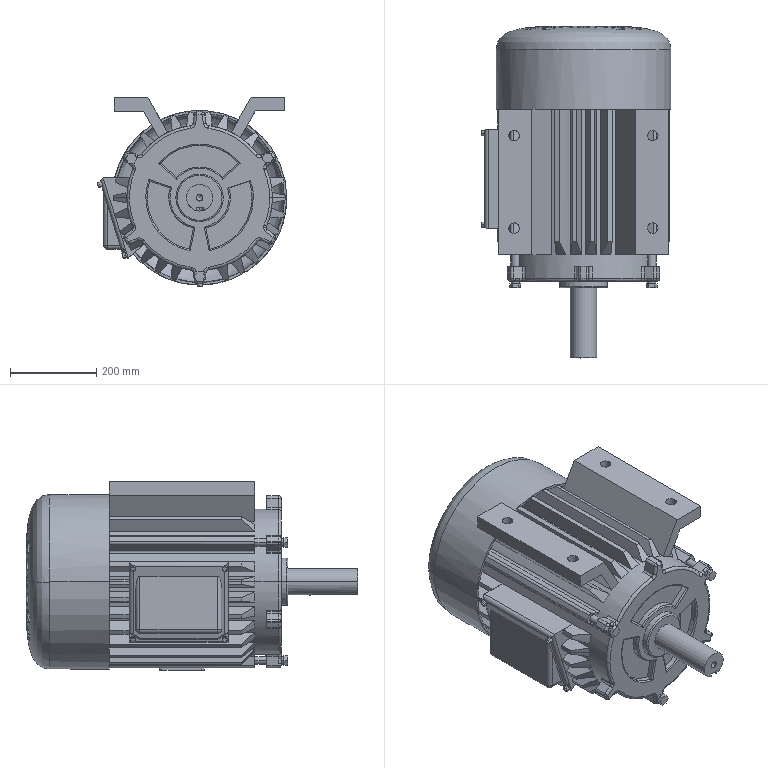Part | NX | features BREP 2, Delete Body 1, EXTRUDE 1, LINKED_FACE 1, REPLACE_FACE 1, SCALE 1, SPLIT BODY 1, UNITE 1 | 1 solid | 624 faces | box 440.662 x 771.03 x 438.512 mm | volume 51845924 mm3 | cylinder 288 | plane 227 | torus 43 | cone 26 | spline 24 | sphere 16 | commonest cylinder face diameters 12.288 x98 30.72 x80 399.36 x39 6.144 x13 18.529 x12 18.432 x9